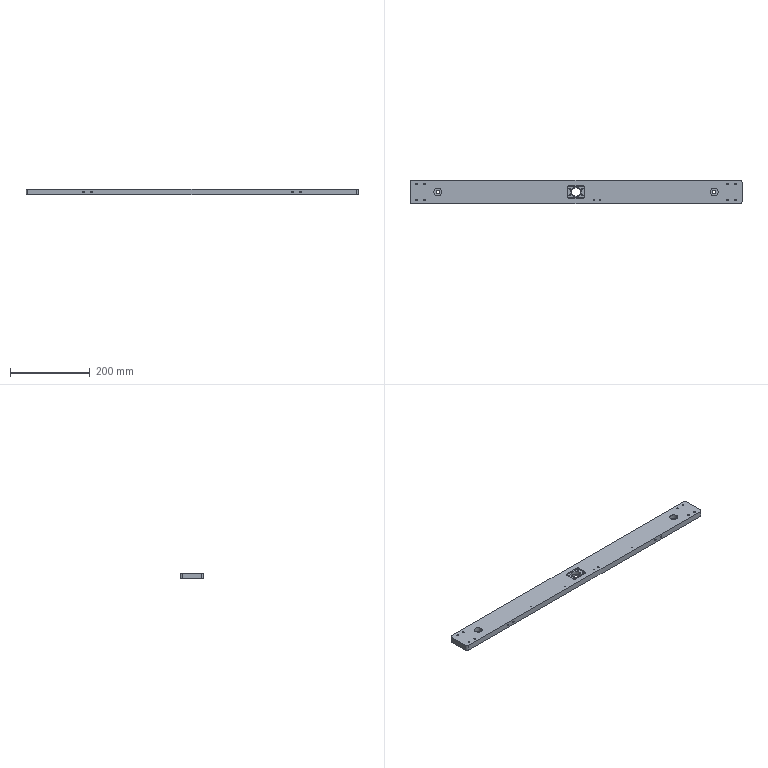Part | STEP file | rear return support plate | 1 solid | 116 faces | box 835 x 60 x 15 mm | volume 730825 mm3 | cylinder 67 | cone 30 | plane 19 | commonest cylinder face diameters 4.2 x24 3.3 x20 4 x7 9 x4 10 x4 20 x4